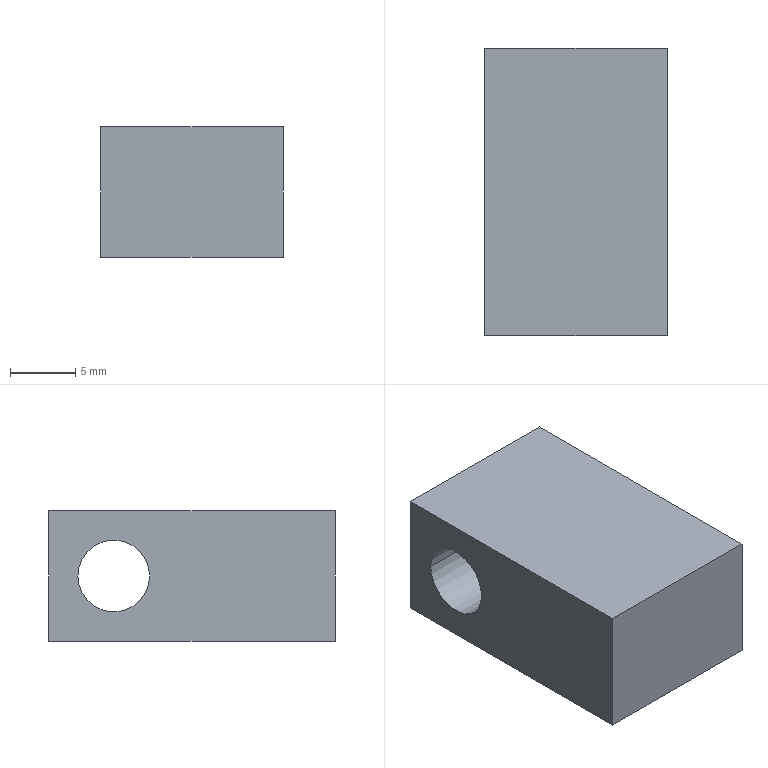Part | NX | 1 solid | 8 faces | box 14 x 22 x 10 mm | volume 2747 mm3 | plane 6 | cylinder 2 | commonest cylinder face diameters 5.5 x2
STEP:
#1=CARTESIAN_POINT('',(606.,86.4,-254.82));
#2=VERTEX_POINT('',#1);
#3=CARTESIAN_POINT('',(606.,86.4,-264.82));
#4=VERTEX_POINT('',#3);
#5=CARTESIAN_POINT('',(606.,86.4,-262.711));
#6=DIRECTION('',(0.,0.,-1.));
#7=VECTOR('',#6,1000.);
#8=LINE('',#5,#7);
#9=EDGE_CURVE('',#2,#4,#8,.T.);
#10=ORIENTED_EDGE('',*,*,#9,.T.);
#11=CARTESIAN_POINT('',(592.,86.4,-264.82));
#12=VERTEX_POINT('',#11);
#13=CARTESIAN_POINT('',(594.,86.4,-264.82));
#14=DIRECTION('',(1.,0.,0.));
#15=VECTOR('',#14,1000.);
#16=LINE('',#13,#15);
#17=EDGE_CURVE('',#12,#4,#16,.T.);
#18=ORIENTED_EDGE('',*,*,#17,.F.);
#19=CARTESIAN_POINT('',(592.,86.4,-254.82));
#20=VERTEX_POINT('',#19);
#21=CARTESIAN_POINT('',(592.,86.4,-262.711));
#22=DIRECTION('',(0.,0.,1.));
#23=VECTOR('',#22,1000.);
#24=LINE('',#21,#23);
#25=EDGE_CURVE('',#12,#20,#24,.T.);
#26=ORIENTED_EDGE('',*,*,#25,.T.);
#27=CARTESIAN_POINT('',(594.,86.4,-254.82));
#28=DIRECTION('',(1.,0.,0.));
#29=VECTOR('',#28,1000.);
#30=LINE('',#27,#29);
#31=EDGE_CURVE('',#20,#2,#30,.T.);
#32=ORIENTED_EDGE('',*,*,#31,.T.);
#33=EDGE_LOOP('',(#10,#18,#26,#32));
#34=FACE_BOUND('',#33,.T.);
#35=CARTESIAN_POINT('',(594.,86.4,-264.82));
#36=DIRECTION('',(0.,1.,0.));
#37=DIRECTION('',(1.,0.,0.));
#38=AXIS2_PLACEMENT_3D('',#35,#36,#37);
#39=PLANE('',#38);
#40=ADVANCED_FACE('',(#34),#39,.T.);
#41=CARTESIAN_POINT('',(606.,64.4,-264.82));
#42=VERTEX_POINT('',#41);
#43=CARTESIAN_POINT('',(606.,82.666,-264.82));
#44=DIRECTION('',(0.,-1.,0.));
#45=VECTOR('',#44,1000.);
#46=LINE('',#43,#45);
#47=EDGE_CURVE('',#4,#42,#46,.T.);
#48=ORIENTED_EDGE('',*,*,#47,.T.);
#49=CARTESIAN_POINT('',(592.,64.4,-264.82));
#50=VERTEX_POINT('',#49);
#51=CARTESIAN_POINT('',(594.,64.4,-264.82));
#52=DIRECTION('',(-1.,0.,0.));
#53=VECTOR('',#52,1000.);
#54=LINE('',#51,#53);
#55=EDGE_CURVE('',#42,#50,#54,.T.);
#56=ORIENTED_EDGE('',*,*,#55,.T.);
#57=CARTESIAN_POINT('',(592.,82.666,-264.82));
#58=DIRECTION('',(0.,1.,0.));
#59=VECTOR('',#58,1000.);
#60=LINE('',#57,#59);
#61=EDGE_CURVE('',#50,#12,#60,.T.);
#62=ORIENTED_EDGE('',*,*,#61,.T.);
#63=ORIENTED_EDGE('',*,*,#17,.T.);
#64=EDGE_LOOP('',(#48,#56,#62,#63));
#65=FACE_BOUND('',#64,.T.);
#66=CARTESIAN_POINT('',(594.,75.9,-264.82));
#67=DIRECTION('',(0.,0.,-1.));
#68=DIRECTION('',(0.,-1.,0.));
#69=AXIS2_PLACEMENT_3D('',#66,#67,#68);
#70=PLANE('',#69);
#71=ADVANCED_FACE('',(#65),#70,.T.);
#72=CARTESIAN_POINT('',(606.,64.4,-254.82));
#73=VERTEX_POINT('',#72);
#74=CARTESIAN_POINT('',(606.,64.4,-262.711));
#75=DIRECTION('',(0.,0.,1.));
#76=VECTOR('',#75,1000.);
#77=LINE('',#74,#76);
#78=EDGE_CURVE('',#42,#73,#77,.T.);
#79=ORIENTED_EDGE('',*,*,#78,.T.);
#80=CARTESIAN_POINT('',(592.,64.4,-254.82));
#81=VERTEX_POINT('',#80);
#82=CARTESIAN_POINT('',(594.,64.4,-254.82));
#83=DIRECTION('',(-1.,0.,0.));
#84=VECTOR('',#83,1000.);
#85=LINE('',#82,#84);
#86=EDGE_CURVE('',#73,#81,#85,.T.);
#87=ORIENTED_EDGE('',*,*,#86,.T.);
#88=CARTESIAN_POINT('',(592.,64.4,-262.711));
#89=DIRECTION('',(0.,0.,-1.));
#90=VECTOR('',#89,1000.);
#91=LINE('',#88,#90);
#92=EDGE_CURVE('',#81,#50,#91,.T.);
#93=ORIENTED_EDGE('',*,*,#92,.T.);
#94=ORIENTED_EDGE('',*,*,#55,.F.);
#95=EDGE_LOOP('',(#79,#87,#93,#94));
#96=FACE_BOUND('',#95,.T.);
#97=CARTESIAN_POINT('',(594.,64.4,-254.82));
#98=DIRECTION('',(0.,-1.,0.));
#99=DIRECTION('',(0.,0.,-1.));
#100=AXIS2_PLACEMENT_3D('',#97,#98,#99);
#101=PLANE('',#100);
#102=ADVANCED_FACE('',(#96),#101,.T.);
#103=CARTESIAN_POINT('',(606.,82.666,-254.82));
#104=DIRECTION('',(0.,-1.,0.));
#105=VECTOR('',#104,1000.);
#106=LINE('',#103,#105);
#107=EDGE_CURVE('',#2,#73,#106,.T.);
#108=ORIENTED_EDGE('',*,*,#107,.F.);
#109=ORIENTED_EDGE('',*,*,#31,.F.);
#110=CARTESIAN_POINT('',(592.,82.666,-254.82));
#111=DIRECTION('',(0.,-1.,0.));
#112=VECTOR('',#111,1000.);
#113=LINE('',#110,#112);
#114=EDGE_CURVE('',#20,#81,#113,.T.);
#115=ORIENTED_EDGE('',*,*,#114,.T.);
#116=ORIENTED_EDGE('',*,*,#86,.F.);
#117=EDGE_LOOP('',(#108,#109,#115,#116));
#118=FACE_BOUND('',#117,.T.);
#119=CARTESIAN_POINT('',(594.,86.9,-254.82));
#120=DIRECTION('',(0.,0.,1.));
#121=DIRECTION('',(1.,0.,0.));
#122=AXIS2_PLACEMENT_3D('',#119,#120,#121);
#123=PLANE('',#122);
#124=ADVANCED_FACE('',(#118),#123,.T.);
#125=CARTESIAN_POINT('',(606.,84.15,-259.82));
#126=VERTEX_POINT('',#125);
#127=CARTESIAN_POINT('',(606.,78.65,-259.82));
#128=VERTEX_POINT('',#127);
#129=CARTESIAN_POINT('',(606.,81.4,-259.82));
#130=DIRECTION('',(1.,0.,0.));
#131=DIRECTION('',(0.,1.,0.));
#132=AXIS2_PLACEMENT_3D('',#129,#130,#131);
#133=CIRCLE('',#132,2.75);
#134=EDGE_CURVE('',#126,#128,#133,.T.);
#135=ORIENTED_EDGE('',*,*,#134,.T.);
#136=CARTESIAN_POINT('',(592.,78.65,-259.82));
#137=VERTEX_POINT('',#136);
#138=CARTESIAN_POINT('',(594.,78.65,-259.82));
#139=DIRECTION('',(1.,0.,0.));
#140=VECTOR('',#139,1000.);
#141=LINE('',#138,#140);
#142=EDGE_CURVE('',#137,#128,#141,.T.);
#143=ORIENTED_EDGE('',*,*,#142,.F.);
#144=CARTESIAN_POINT('',(592.,84.15,-259.82));
#145=VERTEX_POINT('',#144);
#146=CARTESIAN_POINT('',(592.,81.4,-259.82));
#147=DIRECTION('',(1.,0.,0.));
#148=DIRECTION('',(0.,1.,0.));
#149=AXIS2_PLACEMENT_3D('',#146,#147,#148);
#150=CIRCLE('',#149,2.75);
#151=EDGE_CURVE('',#145,#137,#150,.T.);
#152=ORIENTED_EDGE('',*,*,#151,.F.);
#153=CARTESIAN_POINT('',(594.,84.15,-259.82));
#154=DIRECTION('',(1.,0.,0.));
#155=VECTOR('',#154,1000.);
#156=LINE('',#153,#155);
#157=EDGE_CURVE('',#145,#126,#156,.T.);
#158=ORIENTED_EDGE('',*,*,#157,.T.);
#159=EDGE_LOOP('',(#135,#143,#152,#158));
#160=FACE_BOUND('',#159,.T.);
#161=CARTESIAN_POINT('',(594.,81.4,-259.82));
#162=DIRECTION('',(1.,0.,0.));
#163=DIRECTION('',(0.,1.,0.));
#164=AXIS2_PLACEMENT_3D('',#161,#162,#163);
#165=CYLINDRICAL_SURFACE('',#164,2.75);
#166=ADVANCED_FACE('',(#160),#165,.F.);
#167=ORIENTED_EDGE('',*,*,#9,.F.);
#168=ORIENTED_EDGE('',*,*,#107,.T.);
#169=ORIENTED_EDGE('',*,*,#78,.F.);
#170=ORIENTED_EDGE('',*,*,#47,.F.);
#171=EDGE_LOOP('',(#167,#168,#169,#170));
#172=FACE_BOUND('',#171,.T.);
#173=ORIENTED_EDGE('',*,*,#134,.F.);
#174=CARTESIAN_POINT('',(606.,81.4,-259.82));
#175=DIRECTION('',(1.,0.,0.));
#176=DIRECTION('',(0.,1.,0.));
#177=AXIS2_PLACEMENT_3D('',#174,#175,#176);
#178=CIRCLE('',#177,2.75);
#179=EDGE_CURVE('',#128,#126,#178,.T.);
#180=ORIENTED_EDGE('',*,*,#179,.F.);
#181=EDGE_LOOP('',(#173,#180));
#182=FACE_BOUND('',#181,.T.);
#183=CARTESIAN_POINT('',(606.,82.666,-262.711));
#184=DIRECTION('',(1.,0.,0.));
#185=DIRECTION('',(0.,1.,0.));
#186=AXIS2_PLACEMENT_3D('',#183,#184,#185);
#187=PLANE('',#186);
#188=ADVANCED_FACE('',(#172,#182),#187,.T.);
#189=ORIENTED_EDGE('',*,*,#61,.F.);
#190=ORIENTED_EDGE('',*,*,#92,.F.);
#191=ORIENTED_EDGE('',*,*,#114,.F.);
#192=ORIENTED_EDGE('',*,*,#25,.F.);
#193=EDGE_LOOP('',(#189,#190,#191,#192));
#194=FACE_BOUND('',#193,.T.);
#195=ORIENTED_EDGE('',*,*,#151,.T.);
#196=CARTESIAN_POINT('',(592.,81.4,-259.82));
#197=DIRECTION('',(1.,0.,0.));
#198=DIRECTION('',(0.,1.,0.));
#199=AXIS2_PLACEMENT_3D('',#196,#197,#198);
#200=CIRCLE('',#199,2.75);
#201=EDGE_CURVE('',#137,#145,#200,.T.);
#202=ORIENTED_EDGE('',*,*,#201,.T.);
#203=EDGE_LOOP('',(#195,#202));
#204=FACE_BOUND('',#203,.T.);
#205=CARTESIAN_POINT('',(592.,82.666,-262.711));
#206=DIRECTION('',(1.,0.,0.));
#207=DIRECTION('',(0.,1.,0.));
#208=AXIS2_PLACEMENT_3D('',#205,#206,#207);
#209=PLANE('',#208);
#210=ADVANCED_FACE('',(#194,#204),#209,.F.);
#211=ORIENTED_EDGE('',*,*,#157,.F.);
#212=ORIENTED_EDGE('',*,*,#201,.F.);
#213=ORIENTED_EDGE('',*,*,#142,.T.);
#214=ORIENTED_EDGE('',*,*,#179,.T.);
#215=EDGE_LOOP('',(#211,#212,#213,#214));
#216=FACE_BOUND('',#215,.T.);
#217=CARTESIAN_POINT('',(594.,81.4,-259.82));
#218=DIRECTION('',(1.,0.,0.));
#219=DIRECTION('',(0.,1.,0.));
#220=AXIS2_PLACEMENT_3D('',#217,#218,#219);
#221=CYLINDRICAL_SURFACE('',#220,2.75);
#222=ADVANCED_FACE('',(#216),#221,.F.);
#223=CLOSED_SHELL('',(#40,#71,#102,#124,#166,#188,#210,#222));
#224=MANIFOLD_SOLID_BREP('',#223);
#225=(LENGTH_UNIT()NAMED_UNIT(*)SI_UNIT(.MILLI.,.METRE.));
#226=UNCERTAINTY_MEASURE_WITH_UNIT(LENGTH_MEASURE(0.00001),#225,'','');
#227=(NAMED_UNIT(*)PLANE_ANGLE_UNIT()SI_UNIT($,.RADIAN.));
#228=(NAMED_UNIT(*)SI_UNIT($,.STERADIAN.)SOLID_ANGLE_UNIT());
#229=(GEOMETRIC_REPRESENTATION_CONTEXT(3)GLOBAL_UNCERTAINTY_ASSIGNED_CONTEXT((#226))GLOBAL_UNIT_ASSIGNED_CONTEXT((#225,#227,#228))REPRESENTATION_CONTEXT('',''));
#230=ADVANCED_BREP_SHAPE_REPRESENTATION('',(#224),#229);